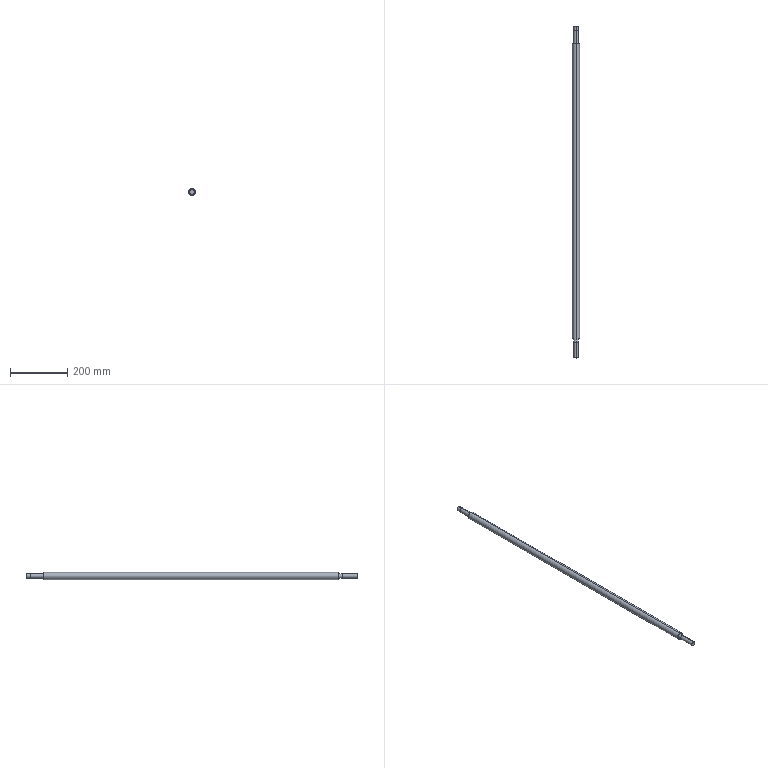Part | SolidWorks | features Revolution 1 | 1 solid | 16 faces | box 25 x 1157 x 25 mm | volume 530644 mm3 | cylinder 10 | plane 6 | commonest cylinder face diameters 15 x4 17 x4 25 x2
STEP:
#1=CARTESIAN_POINT('',(0.,-1102.,-7.5));
#2=VERTEX_POINT('',#1);
#3=CARTESIAN_POINT('',(0.,-1102.,7.5));
#4=VERTEX_POINT('',#3);
#5=CARTESIAN_POINT('',(0.,-1102.,0.));
#6=DIRECTION('',(0.,-1.,0.));
#7=DIRECTION('',(0.,0.,-1.));
#8=AXIS2_PLACEMENT_3D('',#5,#6,#7);
#9=CIRCLE('',#8,7.5);
#10=EDGE_CURVE('',#2,#4,#9,.T.);
#11=ORIENTED_EDGE('',*,*,#10,.T.);
#12=CARTESIAN_POINT('',(0.,-1157.,7.5));
#13=VERTEX_POINT('',#12);
#14=CARTESIAN_POINT('',(0.,0.,7.5));
#15=DIRECTION('',(0.,-1.,0.));
#16=VECTOR('',#15,1000.);
#17=LINE('',#14,#16);
#18=EDGE_CURVE('',#4,#13,#17,.T.);
#19=ORIENTED_EDGE('',*,*,#18,.T.);
#20=CARTESIAN_POINT('',(0.,-1157.,-7.5));
#21=VERTEX_POINT('',#20);
#22=CARTESIAN_POINT('',(0.,-1157.,0.));
#23=DIRECTION('',(0.,-1.,0.));
#24=DIRECTION('',(0.,0.,-1.));
#25=AXIS2_PLACEMENT_3D('',#22,#23,#24);
#26=CIRCLE('',#25,7.5);
#27=EDGE_CURVE('',#21,#13,#26,.T.);
#28=ORIENTED_EDGE('',*,*,#27,.F.);
#29=CARTESIAN_POINT('',(0.,0.,-7.5));
#30=DIRECTION('',(0.,-1.,0.));
#31=VECTOR('',#30,1000.);
#32=LINE('',#29,#31);
#33=EDGE_CURVE('',#2,#21,#32,.T.);
#34=ORIENTED_EDGE('',*,*,#33,.F.);
#35=EDGE_LOOP('',(#11,#19,#28,#34));
#36=FACE_OUTER_BOUND('',#35,.T.);
#37=CARTESIAN_POINT('',(0.,0.,0.));
#38=DIRECTION('',(0.,-1.,0.));
#39=DIRECTION('',(0.,0.,-1.));
#40=AXIS2_PLACEMENT_3D('',#37,#38,#39);
#41=CYLINDRICAL_SURFACE('',#40,7.5);
#42=ADVANCED_FACE('',(#36),#41,.T.);
#43=CARTESIAN_POINT('',(0.,-1090.,-8.5));
#44=VERTEX_POINT('',#43);
#45=CARTESIAN_POINT('',(0.,-1090.,8.5));
#46=VERTEX_POINT('',#45);
#47=CARTESIAN_POINT('',(0.,-1090.,0.));
#48=DIRECTION('',(0.,-1.,0.));
#49=DIRECTION('',(0.,0.,-1.));
#50=AXIS2_PLACEMENT_3D('',#47,#48,#49);
#51=CIRCLE('',#50,8.5);
#52=EDGE_CURVE('',#44,#46,#51,.T.);
#53=ORIENTED_EDGE('',*,*,#52,.T.);
#54=CARTESIAN_POINT('',(0.,-1102.,8.5));
#55=VERTEX_POINT('',#54);
#56=CARTESIAN_POINT('',(0.,0.,8.5));
#57=DIRECTION('',(0.,-1.,0.));
#58=VECTOR('',#57,1000.);
#59=LINE('',#56,#58);
#60=EDGE_CURVE('',#46,#55,#59,.T.);
#61=ORIENTED_EDGE('',*,*,#60,.T.);
#62=CARTESIAN_POINT('',(0.,-1102.,-8.5));
#63=VERTEX_POINT('',#62);
#64=CARTESIAN_POINT('',(0.,-1102.,0.));
#65=DIRECTION('',(0.,-1.,0.));
#66=DIRECTION('',(0.,0.,-1.));
#67=AXIS2_PLACEMENT_3D('',#64,#65,#66);
#68=CIRCLE('',#67,8.5);
#69=EDGE_CURVE('',#63,#55,#68,.T.);
#70=ORIENTED_EDGE('',*,*,#69,.F.);
#71=CARTESIAN_POINT('',(0.,0.,-8.5));
#72=DIRECTION('',(0.,-1.,0.));
#73=VECTOR('',#72,1000.);
#74=LINE('',#71,#73);
#75=EDGE_CURVE('',#44,#63,#74,.T.);
#76=ORIENTED_EDGE('',*,*,#75,.F.);
#77=EDGE_LOOP('',(#53,#61,#70,#76));
#78=FACE_OUTER_BOUND('',#77,.T.);
#79=CARTESIAN_POINT('',(0.,0.,0.));
#80=DIRECTION('',(0.,-1.,0.));
#81=DIRECTION('',(0.,0.,-1.));
#82=AXIS2_PLACEMENT_3D('',#79,#80,#81);
#83=CYLINDRICAL_SURFACE('',#82,8.5);
#84=ADVANCED_FACE('',(#78),#83,.T.);
#85=CARTESIAN_POINT('',(0.,-61.,-12.5));
#86=VERTEX_POINT('',#85);
#87=CARTESIAN_POINT('',(0.,-61.,12.5));
#88=VERTEX_POINT('',#87);
#89=CARTESIAN_POINT('',(0.,-61.,0.));
#90=DIRECTION('',(0.,-1.,0.));
#91=DIRECTION('',(0.,0.,-1.));
#92=AXIS2_PLACEMENT_3D('',#89,#90,#91);
#93=CIRCLE('',#92,12.5);
#94=EDGE_CURVE('',#86,#88,#93,.T.);
#95=ORIENTED_EDGE('',*,*,#94,.T.);
#96=CARTESIAN_POINT('',(0.,-1090.,12.5));
#97=VERTEX_POINT('',#96);
#98=CARTESIAN_POINT('',(0.,0.,12.5));
#99=DIRECTION('',(0.,-1.,0.));
#100=VECTOR('',#99,1000.);
#101=LINE('',#98,#100);
#102=EDGE_CURVE('',#88,#97,#101,.T.);
#103=ORIENTED_EDGE('',*,*,#102,.T.);
#104=CARTESIAN_POINT('',(0.,-1090.,-12.5));
#105=VERTEX_POINT('',#104);
#106=CARTESIAN_POINT('',(0.,-1090.,0.));
#107=DIRECTION('',(0.,-1.,0.));
#108=DIRECTION('',(0.,0.,-1.));
#109=AXIS2_PLACEMENT_3D('',#106,#107,#108);
#110=CIRCLE('',#109,12.5);
#111=EDGE_CURVE('',#105,#97,#110,.T.);
#112=ORIENTED_EDGE('',*,*,#111,.F.);
#113=CARTESIAN_POINT('',(0.,0.,-12.5));
#114=DIRECTION('',(0.,-1.,0.));
#115=VECTOR('',#114,1000.);
#116=LINE('',#113,#115);
#117=EDGE_CURVE('',#86,#105,#116,.T.);
#118=ORIENTED_EDGE('',*,*,#117,.F.);
#119=EDGE_LOOP('',(#95,#103,#112,#118));
#120=FACE_OUTER_BOUND('',#119,.T.);
#121=CARTESIAN_POINT('',(0.,0.,0.));
#122=DIRECTION('',(0.,-1.,0.));
#123=DIRECTION('',(0.,0.,-1.));
#124=AXIS2_PLACEMENT_3D('',#121,#122,#123);
#125=CYLINDRICAL_SURFACE('',#124,12.5);
#126=ADVANCED_FACE('',(#120),#125,.T.);
#127=CARTESIAN_POINT('',(0.,-15.,-8.5));
#128=VERTEX_POINT('',#127);
#129=CARTESIAN_POINT('',(0.,-15.,8.5));
#130=VERTEX_POINT('',#129);
#131=CARTESIAN_POINT('',(0.,-15.,0.));
#132=DIRECTION('',(0.,-1.,0.));
#133=DIRECTION('',(0.,0.,-1.));
#134=AXIS2_PLACEMENT_3D('',#131,#132,#133);
#135=CIRCLE('',#134,8.5);
#136=EDGE_CURVE('',#128,#130,#135,.T.);
#137=ORIENTED_EDGE('',*,*,#136,.T.);
#138=CARTESIAN_POINT('',(0.,-61.,8.5));
#139=VERTEX_POINT('',#138);
#140=CARTESIAN_POINT('',(0.,0.,8.5));
#141=DIRECTION('',(0.,-1.,0.));
#142=VECTOR('',#141,1000.);
#143=LINE('',#140,#142);
#144=EDGE_CURVE('',#130,#139,#143,.T.);
#145=ORIENTED_EDGE('',*,*,#144,.T.);
#146=CARTESIAN_POINT('',(0.,-61.,-8.5));
#147=VERTEX_POINT('',#146);
#148=CARTESIAN_POINT('',(0.,-61.,0.));
#149=DIRECTION('',(0.,-1.,0.));
#150=DIRECTION('',(0.,0.,-1.));
#151=AXIS2_PLACEMENT_3D('',#148,#149,#150);
#152=CIRCLE('',#151,8.5);
#153=EDGE_CURVE('',#147,#139,#152,.T.);
#154=ORIENTED_EDGE('',*,*,#153,.F.);
#155=CARTESIAN_POINT('',(0.,0.,-8.5));
#156=DIRECTION('',(0.,-1.,0.));
#157=VECTOR('',#156,1000.);
#158=LINE('',#155,#157);
#159=EDGE_CURVE('',#128,#147,#158,.T.);
#160=ORIENTED_EDGE('',*,*,#159,.F.);
#161=EDGE_LOOP('',(#137,#145,#154,#160));
#162=FACE_OUTER_BOUND('',#161,.T.);
#163=CARTESIAN_POINT('',(0.,0.,0.));
#164=DIRECTION('',(0.,-1.,0.));
#165=DIRECTION('',(0.,0.,-1.));
#166=AXIS2_PLACEMENT_3D('',#163,#164,#165);
#167=CYLINDRICAL_SURFACE('',#166,8.5);
#168=ADVANCED_FACE('',(#162),#167,.T.);
#169=CARTESIAN_POINT('',(0.,0.,-7.5));
#170=VERTEX_POINT('',#169);
#171=CARTESIAN_POINT('',(0.,0.,7.5));
#172=VERTEX_POINT('',#171);
#173=CARTESIAN_POINT('',(0.,0.,0.));
#174=DIRECTION('',(0.,-1.,0.));
#175=DIRECTION('',(0.,0.,-1.));
#176=AXIS2_PLACEMENT_3D('',#173,#174,#175);
#177=CIRCLE('',#176,7.5);
#178=EDGE_CURVE('',#170,#172,#177,.T.);
#179=ORIENTED_EDGE('',*,*,#178,.T.);
#180=CARTESIAN_POINT('',(0.,-15.,7.5));
#181=VERTEX_POINT('',#180);
#182=CARTESIAN_POINT('',(0.,0.,7.5));
#183=DIRECTION('',(0.,-1.,0.));
#184=VECTOR('',#183,1000.);
#185=LINE('',#182,#184);
#186=EDGE_CURVE('',#172,#181,#185,.T.);
#187=ORIENTED_EDGE('',*,*,#186,.T.);
#188=CARTESIAN_POINT('',(0.,-15.,-7.5));
#189=VERTEX_POINT('',#188);
#190=CARTESIAN_POINT('',(0.,-15.,0.));
#191=DIRECTION('',(0.,-1.,0.));
#192=DIRECTION('',(0.,0.,-1.));
#193=AXIS2_PLACEMENT_3D('',#190,#191,#192);
#194=CIRCLE('',#193,7.5);
#195=EDGE_CURVE('',#189,#181,#194,.T.);
#196=ORIENTED_EDGE('',*,*,#195,.F.);
#197=CARTESIAN_POINT('',(0.,0.,-7.5));
#198=DIRECTION('',(0.,-1.,0.));
#199=VECTOR('',#198,1000.);
#200=LINE('',#197,#199);
#201=EDGE_CURVE('',#170,#189,#200,.T.);
#202=ORIENTED_EDGE('',*,*,#201,.F.);
#203=EDGE_LOOP('',(#179,#187,#196,#202));
#204=FACE_OUTER_BOUND('',#203,.T.);
#205=CARTESIAN_POINT('',(0.,0.,0.));
#206=DIRECTION('',(0.,-1.,0.));
#207=DIRECTION('',(0.,0.,-1.));
#208=AXIS2_PLACEMENT_3D('',#205,#206,#207);
#209=CYLINDRICAL_SURFACE('',#208,7.5);
#210=ADVANCED_FACE('',(#204),#209,.T.);
#211=ORIENTED_EDGE('',*,*,#178,.F.);
#212=CARTESIAN_POINT('',(0.,0.,0.));
#213=DIRECTION('',(0.,-1.,0.));
#214=DIRECTION('',(0.,0.,-1.));
#215=AXIS2_PLACEMENT_3D('',#212,#213,#214);
#216=CIRCLE('',#215,7.5);
#217=EDGE_CURVE('',#172,#170,#216,.T.);
#218=ORIENTED_EDGE('',*,*,#217,.F.);
#219=EDGE_LOOP('',(#211,#218));
#220=FACE_OUTER_BOUND('',#219,.T.);
#221=CARTESIAN_POINT('',(0.,0.,0.));
#222=DIRECTION('',(0.,1.,0.));
#223=DIRECTION('',(0.,0.,1.));
#224=AXIS2_PLACEMENT_3D('',#221,#222,#223);
#225=PLANE('',#224);
#226=ADVANCED_FACE('',(#220),#225,.T.);
#227=ORIENTED_EDGE('',*,*,#186,.F.);
#228=ORIENTED_EDGE('',*,*,#217,.T.);
#229=ORIENTED_EDGE('',*,*,#201,.T.);
#230=CARTESIAN_POINT('',(0.,-15.,0.));
#231=DIRECTION('',(0.,-1.,0.));
#232=DIRECTION('',(0.,0.,-1.));
#233=AXIS2_PLACEMENT_3D('',#230,#231,#232);
#234=CIRCLE('',#233,7.5);
#235=EDGE_CURVE('',#181,#189,#234,.T.);
#236=ORIENTED_EDGE('',*,*,#235,.F.);
#237=EDGE_LOOP('',(#227,#228,#229,#236));
#238=FACE_OUTER_BOUND('',#237,.T.);
#239=CARTESIAN_POINT('',(0.,0.,0.));
#240=DIRECTION('',(0.,-1.,0.));
#241=DIRECTION('',(0.,0.,-1.));
#242=AXIS2_PLACEMENT_3D('',#239,#240,#241);
#243=CYLINDRICAL_SURFACE('',#242,7.5);
#244=ADVANCED_FACE('',(#238),#243,.T.);
#245=ORIENTED_EDGE('',*,*,#195,.T.);
#246=ORIENTED_EDGE('',*,*,#235,.T.);
#247=EDGE_LOOP('',(#245,#246));
#248=FACE_BOUND('',#247,.T.);
#249=ORIENTED_EDGE('',*,*,#136,.F.);
#250=CARTESIAN_POINT('',(0.,-15.,0.));
#251=DIRECTION('',(0.,-1.,0.));
#252=DIRECTION('',(0.,0.,-1.));
#253=AXIS2_PLACEMENT_3D('',#250,#251,#252);
#254=CIRCLE('',#253,8.5);
#255=EDGE_CURVE('',#130,#128,#254,.T.);
#256=ORIENTED_EDGE('',*,*,#255,.F.);
#257=EDGE_LOOP('',(#249,#256));
#258=FACE_OUTER_BOUND('',#257,.T.);
#259=CARTESIAN_POINT('',(7.5,-15.,0.));
#260=DIRECTION('',(0.,1.,0.));
#261=DIRECTION('',(0.,0.,1.));
#262=AXIS2_PLACEMENT_3D('',#259,#260,#261);
#263=PLANE('',#262);
#264=ADVANCED_FACE('',(#248,#258),#263,.T.);
#265=ORIENTED_EDGE('',*,*,#144,.F.);
#266=ORIENTED_EDGE('',*,*,#255,.T.);
#267=ORIENTED_EDGE('',*,*,#159,.T.);
#268=CARTESIAN_POINT('',(0.,-61.,0.));
#269=DIRECTION('',(0.,-1.,0.));
#270=DIRECTION('',(0.,0.,-1.));
#271=AXIS2_PLACEMENT_3D('',#268,#269,#270);
#272=CIRCLE('',#271,8.5);
#273=EDGE_CURVE('',#139,#147,#272,.T.);
#274=ORIENTED_EDGE('',*,*,#273,.F.);
#275=EDGE_LOOP('',(#265,#266,#267,#274));
#276=FACE_OUTER_BOUND('',#275,.T.);
#277=CARTESIAN_POINT('',(0.,0.,0.));
#278=DIRECTION('',(0.,-1.,0.));
#279=DIRECTION('',(0.,0.,-1.));
#280=AXIS2_PLACEMENT_3D('',#277,#278,#279);
#281=CYLINDRICAL_SURFACE('',#280,8.5);
#282=ADVANCED_FACE('',(#276),#281,.T.);
#283=ORIENTED_EDGE('',*,*,#153,.T.);
#284=ORIENTED_EDGE('',*,*,#273,.T.);
#285=EDGE_LOOP('',(#283,#284));
#286=FACE_BOUND('',#285,.T.);
#287=ORIENTED_EDGE('',*,*,#94,.F.);
#288=CARTESIAN_POINT('',(0.,-61.,0.));
#289=DIRECTION('',(0.,-1.,0.));
#290=DIRECTION('',(0.,0.,-1.));
#291=AXIS2_PLACEMENT_3D('',#288,#289,#290);
#292=CIRCLE('',#291,12.5);
#293=EDGE_CURVE('',#88,#86,#292,.T.);
#294=ORIENTED_EDGE('',*,*,#293,.F.);
#295=EDGE_LOOP('',(#287,#294));
#296=FACE_OUTER_BOUND('',#295,.T.);
#297=CARTESIAN_POINT('',(8.5,-61.,0.));
#298=DIRECTION('',(0.,1.,0.));
#299=DIRECTION('',(0.,0.,1.));
#300=AXIS2_PLACEMENT_3D('',#297,#298,#299);
#301=PLANE('',#300);
#302=ADVANCED_FACE('',(#286,#296),#301,.T.);
#303=ORIENTED_EDGE('',*,*,#102,.F.);
#304=ORIENTED_EDGE('',*,*,#293,.T.);
#305=ORIENTED_EDGE('',*,*,#117,.T.);
#306=CARTESIAN_POINT('',(0.,-1090.,0.));
#307=DIRECTION('',(0.,-1.,0.));
#308=DIRECTION('',(0.,0.,-1.));
#309=AXIS2_PLACEMENT_3D('',#306,#307,#308);
#310=CIRCLE('',#309,12.5);
#311=EDGE_CURVE('',#97,#105,#310,.T.);
#312=ORIENTED_EDGE('',*,*,#311,.F.);
#313=EDGE_LOOP('',(#303,#304,#305,#312));
#314=FACE_OUTER_BOUND('',#313,.T.);
#315=CARTESIAN_POINT('',(0.,0.,0.));
#316=DIRECTION('',(0.,-1.,0.));
#317=DIRECTION('',(0.,0.,-1.));
#318=AXIS2_PLACEMENT_3D('',#315,#316,#317);
#319=CYLINDRICAL_SURFACE('',#318,12.5);
#320=ADVANCED_FACE('',(#314),#319,.T.);
#321=ORIENTED_EDGE('',*,*,#111,.T.);
#322=ORIENTED_EDGE('',*,*,#311,.T.);
#323=EDGE_LOOP('',(#321,#322));
#324=FACE_OUTER_BOUND('',#323,.T.);
#325=ORIENTED_EDGE('',*,*,#52,.F.);
#326=CARTESIAN_POINT('',(0.,-1090.,0.));
#327=DIRECTION('',(0.,-1.,0.));
#328=DIRECTION('',(0.,0.,-1.));
#329=AXIS2_PLACEMENT_3D('',#326,#327,#328);
#330=CIRCLE('',#329,8.5);
#331=EDGE_CURVE('',#46,#44,#330,.T.);
#332=ORIENTED_EDGE('',*,*,#331,.F.);
#333=EDGE_LOOP('',(#325,#332));
#334=FACE_BOUND('',#333,.T.);
#335=CARTESIAN_POINT('',(12.5,-1090.,0.));
#336=DIRECTION('',(0.,-1.,0.));
#337=DIRECTION('',(0.,0.,-1.));
#338=AXIS2_PLACEMENT_3D('',#335,#336,#337);
#339=PLANE('',#338);
#340=ADVANCED_FACE('',(#324,#334),#339,.T.);
#341=ORIENTED_EDGE('',*,*,#60,.F.);
#342=ORIENTED_EDGE('',*,*,#331,.T.);
#343=ORIENTED_EDGE('',*,*,#75,.T.);
#344=CARTESIAN_POINT('',(0.,-1102.,0.));
#345=DIRECTION('',(0.,-1.,0.));
#346=DIRECTION('',(0.,0.,-1.));
#347=AXIS2_PLACEMENT_3D('',#344,#345,#346);
#348=CIRCLE('',#347,8.5);
#349=EDGE_CURVE('',#55,#63,#348,.T.);
#350=ORIENTED_EDGE('',*,*,#349,.F.);
#351=EDGE_LOOP('',(#341,#342,#343,#350));
#352=FACE_OUTER_BOUND('',#351,.T.);
#353=CARTESIAN_POINT('',(0.,0.,0.));
#354=DIRECTION('',(0.,-1.,0.));
#355=DIRECTION('',(0.,0.,-1.));
#356=AXIS2_PLACEMENT_3D('',#353,#354,#355);
#357=CYLINDRICAL_SURFACE('',#356,8.5);
#358=ADVANCED_FACE('',(#352),#357,.T.);
#359=ORIENTED_EDGE('',*,*,#69,.T.);
#360=ORIENTED_EDGE('',*,*,#349,.T.);
#361=EDGE_LOOP('',(#359,#360));
#362=FACE_OUTER_BOUND('',#361,.T.);
#363=ORIENTED_EDGE('',*,*,#10,.F.);
#364=CARTESIAN_POINT('',(0.,-1102.,0.));
#365=DIRECTION('',(0.,-1.,0.));
#366=DIRECTION('',(0.,0.,-1.));
#367=AXIS2_PLACEMENT_3D('',#364,#365,#366);
#368=CIRCLE('',#367,7.5);
#369=EDGE_CURVE('',#4,#2,#368,.T.);
#370=ORIENTED_EDGE('',*,*,#369,.F.);
#371=EDGE_LOOP('',(#363,#370));
#372=FACE_BOUND('',#371,.T.);
#373=CARTESIAN_POINT('',(8.5,-1102.,0.));
#374=DIRECTION('',(0.,-1.,0.));
#375=DIRECTION('',(0.,0.,-1.));
#376=AXIS2_PLACEMENT_3D('',#373,#374,#375);
#377=PLANE('',#376);
#378=ADVANCED_FACE('',(#362,#372),#377,.T.);
#379=ORIENTED_EDGE('',*,*,#18,.F.);
#380=ORIENTED_EDGE('',*,*,#369,.T.);
#381=ORIENTED_EDGE('',*,*,#33,.T.);
#382=CARTESIAN_POINT('',(0.,-1157.,0.));
#383=DIRECTION('',(0.,-1.,0.));
#384=DIRECTION('',(0.,0.,-1.));
#385=AXIS2_PLACEMENT_3D('',#382,#383,#384);
#386=CIRCLE('',#385,7.5);
#387=EDGE_CURVE('',#13,#21,#386,.T.);
#388=ORIENTED_EDGE('',*,*,#387,.F.);
#389=EDGE_LOOP('',(#379,#380,#381,#388));
#390=FACE_OUTER_BOUND('',#389,.T.);
#391=CARTESIAN_POINT('',(0.,0.,0.));
#392=DIRECTION('',(0.,-1.,0.));
#393=DIRECTION('',(0.,0.,-1.));
#394=AXIS2_PLACEMENT_3D('',#391,#392,#393);
#395=CYLINDRICAL_SURFACE('',#394,7.5);
#396=ADVANCED_FACE('',(#390),#395,.T.);
#397=ORIENTED_EDGE('',*,*,#27,.T.);
#398=ORIENTED_EDGE('',*,*,#387,.T.);
#399=EDGE_LOOP('',(#397,#398));
#400=FACE_OUTER_BOUND('',#399,.T.);
#401=CARTESIAN_POINT('',(7.5,-1157.,0.));
#402=DIRECTION('',(0.,-1.,0.));
#403=DIRECTION('',(0.,0.,-1.));
#404=AXIS2_PLACEMENT_3D('',#401,#402,#403);
#405=PLANE('',#404);
#406=ADVANCED_FACE('',(#400),#405,.T.);
#407=CLOSED_SHELL('',(#42,#84,#126,#168,#210,#226,#244,#264,#282,#302,#320,#340,#358,#378,#396,#406));
#408=MANIFOLD_SOLID_BREP('',#407);
#409=CARTESIAN_POINT('',(0.,0.,0.));
#410=DIRECTION('',(0.,0.,1.));
#411=DIRECTION('',(1.,0.,0.));
#412=AXIS2_PLACEMENT_3D('',#409,#410,#411);
#413=(LENGTH_UNIT()NAMED_UNIT(*)SI_UNIT(.MILLI.,.METRE.));
#414=UNCERTAINTY_MEASURE_WITH_UNIT(LENGTH_MEASURE(0.00001),#413,'','');
#415=(NAMED_UNIT(*)PLANE_ANGLE_UNIT()SI_UNIT($,.RADIAN.));
#416=(NAMED_UNIT(*)SI_UNIT($,.STERADIAN.)SOLID_ANGLE_UNIT());
#417=(GEOMETRIC_REPRESENTATION_CONTEXT(3)GLOBAL_UNCERTAINTY_ASSIGNED_CONTEXT((#414))GLOBAL_UNIT_ASSIGNED_CONTEXT((#413,#415,#416))REPRESENTATION_CONTEXT('',''));
#418=ADVANCED_BREP_SHAPE_REPRESENTATION('',(#408,#412),#417);